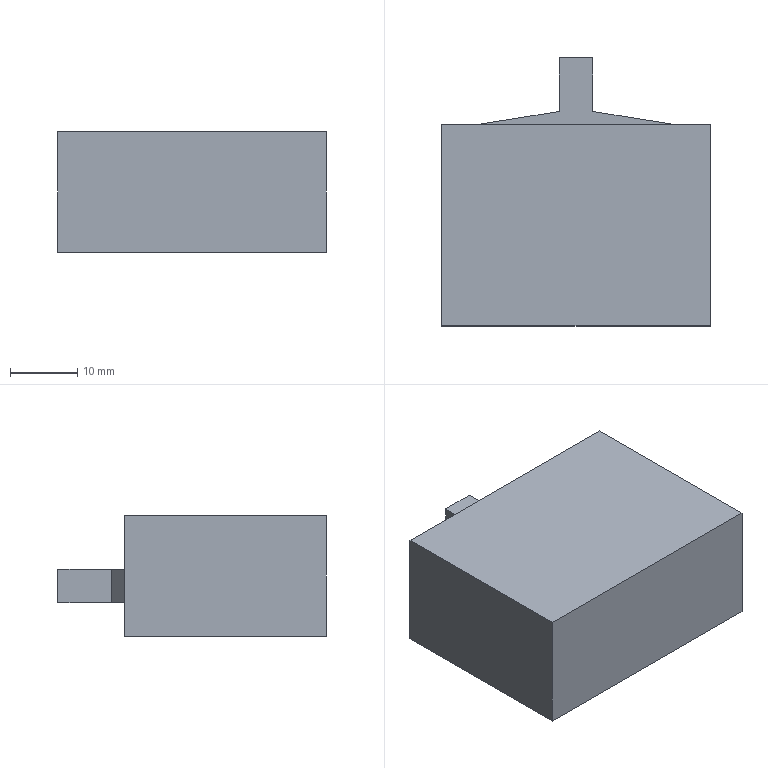Part | SolidWorks | features Extrusion 1, ICE 1 | 1 solid | 13 faces | box 40 x 40 x 18 mm | volume 21975 mm3 | plane 13
STEP:
#1=CARTESIAN_POINT('',(0.,0.,0.));
#2=VERTEX_POINT('',#1);
#3=CARTESIAN_POINT('',(0.,-30.,0.));
#4=VERTEX_POINT('',#3);
#5=CARTESIAN_POINT('',(0.,0.,0.));
#6=DIRECTION('',(0.,-1.,0.));
#7=VECTOR('',#6,1000.);
#8=LINE('',#5,#7);
#9=EDGE_CURVE('',#2,#4,#8,.T.);
#10=ORIENTED_EDGE('',*,*,#9,.T.);
#11=CARTESIAN_POINT('',(0.,-30.,18.));
#12=VERTEX_POINT('',#11);
#13=CARTESIAN_POINT('',(0.,-30.,18.));
#14=DIRECTION('',(0.,0.,-1.));
#15=VECTOR('',#14,1000.);
#16=LINE('',#13,#15);
#17=EDGE_CURVE('',#12,#4,#16,.T.);
#18=ORIENTED_EDGE('',*,*,#17,.F.);
#19=CARTESIAN_POINT('',(0.,0.,18.));
#20=VERTEX_POINT('',#19);
#21=CARTESIAN_POINT('',(0.,0.,18.));
#22=DIRECTION('',(0.,-1.,0.));
#23=VECTOR('',#22,1000.);
#24=LINE('',#21,#23);
#25=EDGE_CURVE('',#20,#12,#24,.T.);
#26=ORIENTED_EDGE('',*,*,#25,.F.);
#27=CARTESIAN_POINT('',(0.,0.,18.));
#28=DIRECTION('',(0.,0.,-1.));
#29=VECTOR('',#28,1000.);
#30=LINE('',#27,#29);
#31=EDGE_CURVE('',#20,#2,#30,.T.);
#32=ORIENTED_EDGE('',*,*,#31,.T.);
#33=EDGE_LOOP('',(#10,#18,#26,#32));
#34=FACE_OUTER_BOUND('',#33,.T.);
#35=CARTESIAN_POINT('',(0.,0.,18.));
#36=DIRECTION('',(1.,0.,0.));
#37=DIRECTION('',(0.,1.,0.));
#38=AXIS2_PLACEMENT_3D('',#35,#36,#37);
#39=PLANE('',#38);
#40=ADVANCED_FACE('',(#34),#39,.F.);
#41=CARTESIAN_POINT('',(40.,-30.,0.));
#42=VERTEX_POINT('',#41);
#43=CARTESIAN_POINT('',(0.,-30.,0.));
#44=DIRECTION('',(1.,0.,0.));
#45=VECTOR('',#44,1000.);
#46=LINE('',#43,#45);
#47=EDGE_CURVE('',#4,#42,#46,.T.);
#48=ORIENTED_EDGE('',*,*,#47,.T.);
#49=CARTESIAN_POINT('',(40.,-30.,18.));
#50=VERTEX_POINT('',#49);
#51=CARTESIAN_POINT('',(40.,-30.,18.));
#52=DIRECTION('',(0.,0.,-1.));
#53=VECTOR('',#52,1000.);
#54=LINE('',#51,#53);
#55=EDGE_CURVE('',#50,#42,#54,.T.);
#56=ORIENTED_EDGE('',*,*,#55,.F.);
#57=CARTESIAN_POINT('',(0.,-30.,18.));
#58=DIRECTION('',(1.,0.,0.));
#59=VECTOR('',#58,1000.);
#60=LINE('',#57,#59);
#61=EDGE_CURVE('',#12,#50,#60,.T.);
#62=ORIENTED_EDGE('',*,*,#61,.F.);
#63=ORIENTED_EDGE('',*,*,#17,.T.);
#64=EDGE_LOOP('',(#48,#56,#62,#63));
#65=FACE_OUTER_BOUND('',#64,.T.);
#66=CARTESIAN_POINT('',(0.,-30.,18.));
#67=DIRECTION('',(0.,1.,0.));
#68=DIRECTION('',(0.,0.,1.));
#69=AXIS2_PLACEMENT_3D('',#66,#67,#68);
#70=PLANE('',#69);
#71=ADVANCED_FACE('',(#65),#70,.F.);
#72=CARTESIAN_POINT('',(40.,0.,0.));
#73=VERTEX_POINT('',#72);
#74=CARTESIAN_POINT('',(40.,0.,0.));
#75=DIRECTION('',(0.,1.,0.));
#76=VECTOR('',#75,1000.);
#77=LINE('',#74,#76);
#78=EDGE_CURVE('',#42,#73,#77,.T.);
#79=ORIENTED_EDGE('',*,*,#78,.T.);
#80=CARTESIAN_POINT('',(40.,0.,18.));
#81=VERTEX_POINT('',#80);
#82=CARTESIAN_POINT('',(40.,0.,18.));
#83=DIRECTION('',(0.,0.,-1.));
#84=VECTOR('',#83,1000.);
#85=LINE('',#82,#84);
#86=EDGE_CURVE('',#81,#73,#85,.T.);
#87=ORIENTED_EDGE('',*,*,#86,.F.);
#88=CARTESIAN_POINT('',(40.,0.,18.));
#89=DIRECTION('',(0.,1.,0.));
#90=VECTOR('',#89,1000.);
#91=LINE('',#88,#90);
#92=EDGE_CURVE('',#50,#81,#91,.T.);
#93=ORIENTED_EDGE('',*,*,#92,.F.);
#94=ORIENTED_EDGE('',*,*,#55,.T.);
#95=EDGE_LOOP('',(#79,#87,#93,#94));
#96=FACE_OUTER_BOUND('',#95,.T.);
#97=CARTESIAN_POINT('',(40.,0.,18.));
#98=DIRECTION('',(-1.,0.,0.));
#99=DIRECTION('',(0.,-1.,0.));
#100=AXIS2_PLACEMENT_3D('',#97,#98,#99);
#101=PLANE('',#100);
#102=ADVANCED_FACE('',(#96),#101,.F.);
#103=CARTESIAN_POINT('',(5.,0.,10.));
#104=VERTEX_POINT('',#103);
#105=CARTESIAN_POINT('',(5.,0.,5.));
#106=VERTEX_POINT('',#105);
#107=CARTESIAN_POINT('',(5.,0.,10.));
#108=DIRECTION('',(0.,0.,-1.));
#109=VECTOR('',#108,1000.);
#110=LINE('',#107,#109);
#111=EDGE_CURVE('',#104,#106,#110,.T.);
#112=ORIENTED_EDGE('',*,*,#111,.T.);
#113=CARTESIAN_POINT('',(35.,0.,5.));
#114=VERTEX_POINT('',#113);
#115=CARTESIAN_POINT('',(0.,0.,5.));
#116=DIRECTION('',(1.,0.,0.));
#117=VECTOR('',#116,1000.);
#118=LINE('',#115,#117);
#119=EDGE_CURVE('',#106,#114,#118,.T.);
#120=ORIENTED_EDGE('',*,*,#119,.T.);
#121=CARTESIAN_POINT('',(35.,0.,10.));
#122=VERTEX_POINT('',#121);
#123=CARTESIAN_POINT('',(35.,0.,10.));
#124=DIRECTION('',(0.,0.,-1.));
#125=VECTOR('',#124,1000.);
#126=LINE('',#123,#125);
#127=EDGE_CURVE('',#122,#114,#126,.T.);
#128=ORIENTED_EDGE('',*,*,#127,.F.);
#129=CARTESIAN_POINT('',(0.,0.,10.));
#130=DIRECTION('',(1.,0.,0.));
#131=VECTOR('',#130,1000.);
#132=LINE('',#129,#131);
#133=EDGE_CURVE('',#104,#122,#132,.T.);
#134=ORIENTED_EDGE('',*,*,#133,.F.);
#135=EDGE_LOOP('',(#112,#120,#128,#134));
#136=FACE_BOUND('',#135,.T.);
#137=CARTESIAN_POINT('',(0.,0.,0.));
#138=DIRECTION('',(-1.,0.,0.));
#139=VECTOR('',#138,1000.);
#140=LINE('',#137,#139);
#141=EDGE_CURVE('',#73,#2,#140,.T.);
#142=ORIENTED_EDGE('',*,*,#141,.T.);
#143=ORIENTED_EDGE('',*,*,#31,.F.);
#144=CARTESIAN_POINT('',(0.,0.,18.));
#145=DIRECTION('',(-1.,0.,0.));
#146=VECTOR('',#145,1000.);
#147=LINE('',#144,#146);
#148=EDGE_CURVE('',#81,#20,#147,.T.);
#149=ORIENTED_EDGE('',*,*,#148,.F.);
#150=ORIENTED_EDGE('',*,*,#86,.T.);
#151=EDGE_LOOP('',(#142,#143,#149,#150));
#152=FACE_OUTER_BOUND('',#151,.T.);
#153=CARTESIAN_POINT('',(0.,0.,18.));
#154=DIRECTION('',(0.,-1.,0.));
#155=DIRECTION('',(0.,0.,-1.));
#156=AXIS2_PLACEMENT_3D('',#153,#154,#155);
#157=PLANE('',#156);
#158=ADVANCED_FACE('',(#136,#152),#157,.F.);
#159=ORIENTED_EDGE('',*,*,#25,.T.);
#160=ORIENTED_EDGE('',*,*,#61,.T.);
#161=ORIENTED_EDGE('',*,*,#92,.T.);
#162=ORIENTED_EDGE('',*,*,#148,.T.);
#163=EDGE_LOOP('',(#159,#160,#161,#162));
#164=FACE_OUTER_BOUND('',#163,.T.);
#165=CARTESIAN_POINT('',(0.,0.,18.));
#166=DIRECTION('',(0.,0.,1.));
#167=DIRECTION('',(1.,0.,0.));
#168=AXIS2_PLACEMENT_3D('',#165,#166,#167);
#169=PLANE('',#168);
#170=ADVANCED_FACE('',(#164),#169,.T.);
#171=ORIENTED_EDGE('',*,*,#9,.F.);
#172=ORIENTED_EDGE('',*,*,#141,.F.);
#173=ORIENTED_EDGE('',*,*,#78,.F.);
#174=ORIENTED_EDGE('',*,*,#47,.F.);
#175=EDGE_LOOP('',(#171,#172,#173,#174));
#176=FACE_OUTER_BOUND('',#175,.T.);
#177=CARTESIAN_POINT('',(0.,0.,0.));
#178=DIRECTION('',(0.,0.,1.));
#179=DIRECTION('',(1.,0.,0.));
#180=AXIS2_PLACEMENT_3D('',#177,#178,#179);
#181=PLANE('',#180);
#182=ADVANCED_FACE('',(#176),#181,.F.);
#183=CARTESIAN_POINT('',(17.5,2.,5.));
#184=VERTEX_POINT('',#183);
#185=CARTESIAN_POINT('',(0.1248,-0.78,5.));
#186=DIRECTION('',(-0.9874,-0.158,0.));
#187=VECTOR('',#186,1000.);
#188=LINE('',#185,#187);
#189=EDGE_CURVE('',#184,#106,#188,.T.);
#190=ORIENTED_EDGE('',*,*,#189,.T.);
#191=ORIENTED_EDGE('',*,*,#111,.F.);
#192=CARTESIAN_POINT('',(17.5,2.,10.));
#193=VERTEX_POINT('',#192);
#194=CARTESIAN_POINT('',(0.1248,-0.78,10.));
#195=DIRECTION('',(-0.9874,-0.158,0.));
#196=VECTOR('',#195,1000.);
#197=LINE('',#194,#196);
#198=EDGE_CURVE('',#193,#104,#197,.T.);
#199=ORIENTED_EDGE('',*,*,#198,.F.);
#200=CARTESIAN_POINT('',(17.5,2.,10.));
#201=DIRECTION('',(0.,0.,-1.));
#202=VECTOR('',#201,1000.);
#203=LINE('',#200,#202);
#204=EDGE_CURVE('',#193,#184,#203,.T.);
#205=ORIENTED_EDGE('',*,*,#204,.T.);
#206=EDGE_LOOP('',(#190,#191,#199,#205));
#207=FACE_OUTER_BOUND('',#206,.T.);
#208=CARTESIAN_POINT('',(0.1248,-0.78,10.));
#209=DIRECTION('',(0.158,-0.9874,0.));
#210=DIRECTION('',(0.9874,0.158,0.));
#211=AXIS2_PLACEMENT_3D('',#208,#209,#210);
#212=PLANE('',#211);
#213=ADVANCED_FACE('',(#207),#212,.F.);
#214=CARTESIAN_POINT('',(22.5,2.,5.));
#215=VERTEX_POINT('',#214);
#216=CARTESIAN_POINT('',(0.8736,5.46,5.));
#217=DIRECTION('',(0.9874,-0.158,0.));
#218=VECTOR('',#217,1000.);
#219=LINE('',#216,#218);
#220=EDGE_CURVE('',#215,#114,#219,.T.);
#221=ORIENTED_EDGE('',*,*,#220,.F.);
#222=CARTESIAN_POINT('',(22.5,2.,10.));
#223=VERTEX_POINT('',#222);
#224=CARTESIAN_POINT('',(22.5,2.,10.));
#225=DIRECTION('',(0.,0.,-1.));
#226=VECTOR('',#225,1000.);
#227=LINE('',#224,#226);
#228=EDGE_CURVE('',#223,#215,#227,.T.);
#229=ORIENTED_EDGE('',*,*,#228,.F.);
#230=CARTESIAN_POINT('',(0.8736,5.46,10.));
#231=DIRECTION('',(0.9874,-0.158,0.));
#232=VECTOR('',#231,1000.);
#233=LINE('',#230,#232);
#234=EDGE_CURVE('',#223,#122,#233,.T.);
#235=ORIENTED_EDGE('',*,*,#234,.T.);
#236=ORIENTED_EDGE('',*,*,#127,.T.);
#237=EDGE_LOOP('',(#221,#229,#235,#236));
#238=FACE_OUTER_BOUND('',#237,.T.);
#239=CARTESIAN_POINT('',(0.8736,5.46,10.));
#240=DIRECTION('',(0.158,0.9874,0.));
#241=DIRECTION('',(-0.9874,0.158,0.));
#242=AXIS2_PLACEMENT_3D('',#239,#240,#241);
#243=PLANE('',#242);
#244=ADVANCED_FACE('',(#238),#243,.T.);
#245=CARTESIAN_POINT('',(22.5,10.,5.));
#246=VERTEX_POINT('',#245);
#247=CARTESIAN_POINT('',(22.5,0.,5.));
#248=DIRECTION('',(0.,1.,0.));
#249=VECTOR('',#248,1000.);
#250=LINE('',#247,#249);
#251=EDGE_CURVE('',#215,#246,#250,.T.);
#252=ORIENTED_EDGE('',*,*,#251,.T.);
#253=CARTESIAN_POINT('',(22.5,10.,10.));
#254=VERTEX_POINT('',#253);
#255=CARTESIAN_POINT('',(22.5,10.,10.));
#256=DIRECTION('',(0.,0.,-1.));
#257=VECTOR('',#256,1000.);
#258=LINE('',#255,#257);
#259=EDGE_CURVE('',#254,#246,#258,.T.);
#260=ORIENTED_EDGE('',*,*,#259,.F.);
#261=CARTESIAN_POINT('',(22.5,0.,10.));
#262=DIRECTION('',(0.,1.,0.));
#263=VECTOR('',#262,1000.);
#264=LINE('',#261,#263);
#265=EDGE_CURVE('',#223,#254,#264,.T.);
#266=ORIENTED_EDGE('',*,*,#265,.F.);
#267=ORIENTED_EDGE('',*,*,#228,.T.);
#268=EDGE_LOOP('',(#252,#260,#266,#267));
#269=FACE_OUTER_BOUND('',#268,.T.);
#270=CARTESIAN_POINT('',(22.5,0.,10.));
#271=DIRECTION('',(-1.,0.,0.));
#272=DIRECTION('',(0.,-1.,0.));
#273=AXIS2_PLACEMENT_3D('',#270,#271,#272);
#274=PLANE('',#273);
#275=ADVANCED_FACE('',(#269),#274,.F.);
#276=CARTESIAN_POINT('',(17.5,10.,5.));
#277=VERTEX_POINT('',#276);
#278=CARTESIAN_POINT('',(0.,10.,5.));
#279=DIRECTION('',(-1.,0.,0.));
#280=VECTOR('',#279,1000.);
#281=LINE('',#278,#280);
#282=EDGE_CURVE('',#246,#277,#281,.T.);
#283=ORIENTED_EDGE('',*,*,#282,.T.);
#284=CARTESIAN_POINT('',(17.5,10.,10.));
#285=VERTEX_POINT('',#284);
#286=CARTESIAN_POINT('',(17.5,10.,10.));
#287=DIRECTION('',(0.,0.,-1.));
#288=VECTOR('',#287,1000.);
#289=LINE('',#286,#288);
#290=EDGE_CURVE('',#285,#277,#289,.T.);
#291=ORIENTED_EDGE('',*,*,#290,.F.);
#292=CARTESIAN_POINT('',(0.,10.,10.));
#293=DIRECTION('',(-1.,0.,0.));
#294=VECTOR('',#293,1000.);
#295=LINE('',#292,#294);
#296=EDGE_CURVE('',#254,#285,#295,.T.);
#297=ORIENTED_EDGE('',*,*,#296,.F.);
#298=ORIENTED_EDGE('',*,*,#259,.T.);
#299=EDGE_LOOP('',(#283,#291,#297,#298));
#300=FACE_OUTER_BOUND('',#299,.T.);
#301=CARTESIAN_POINT('',(0.,10.,10.));
#302=DIRECTION('',(0.,-1.,0.));
#303=DIRECTION('',(0.,0.,-1.));
#304=AXIS2_PLACEMENT_3D('',#301,#302,#303);
#305=PLANE('',#304);
#306=ADVANCED_FACE('',(#300),#305,.F.);
#307=CARTESIAN_POINT('',(17.5,0.,5.));
#308=DIRECTION('',(0.,-1.,0.));
#309=VECTOR('',#308,1000.);
#310=LINE('',#307,#309);
#311=EDGE_CURVE('',#277,#184,#310,.T.);
#312=ORIENTED_EDGE('',*,*,#311,.T.);
#313=ORIENTED_EDGE('',*,*,#204,.F.);
#314=CARTESIAN_POINT('',(17.5,0.,10.));
#315=DIRECTION('',(0.,-1.,0.));
#316=VECTOR('',#315,1000.);
#317=LINE('',#314,#316);
#318=EDGE_CURVE('',#285,#193,#317,.T.);
#319=ORIENTED_EDGE('',*,*,#318,.F.);
#320=ORIENTED_EDGE('',*,*,#290,.T.);
#321=EDGE_LOOP('',(#312,#313,#319,#320));
#322=FACE_OUTER_BOUND('',#321,.T.);
#323=CARTESIAN_POINT('',(17.5,0.,10.));
#324=DIRECTION('',(1.,0.,0.));
#325=DIRECTION('',(0.,1.,0.));
#326=AXIS2_PLACEMENT_3D('',#323,#324,#325);
#327=PLANE('',#326);
#328=ADVANCED_FACE('',(#322),#327,.F.);
#329=ORIENTED_EDGE('',*,*,#198,.T.);
#330=ORIENTED_EDGE('',*,*,#133,.T.);
#331=ORIENTED_EDGE('',*,*,#234,.F.);
#332=ORIENTED_EDGE('',*,*,#265,.T.);
#333=ORIENTED_EDGE('',*,*,#296,.T.);
#334=ORIENTED_EDGE('',*,*,#318,.T.);
#335=EDGE_LOOP('',(#329,#330,#331,#332,#333,#334));
#336=FACE_OUTER_BOUND('',#335,.T.);
#337=CARTESIAN_POINT('',(0.,0.,10.));
#338=DIRECTION('',(0.,0.,-1.));
#339=DIRECTION('',(-1.,0.,0.));
#340=AXIS2_PLACEMENT_3D('',#337,#338,#339);
#341=PLANE('',#340);
#342=ADVANCED_FACE('',(#336),#341,.F.);
#343=ORIENTED_EDGE('',*,*,#189,.F.);
#344=ORIENTED_EDGE('',*,*,#311,.F.);
#345=ORIENTED_EDGE('',*,*,#282,.F.);
#346=ORIENTED_EDGE('',*,*,#251,.F.);
#347=ORIENTED_EDGE('',*,*,#220,.T.);
#348=ORIENTED_EDGE('',*,*,#119,.F.);
#349=EDGE_LOOP('',(#343,#344,#345,#346,#347,#348));
#350=FACE_OUTER_BOUND('',#349,.T.);
#351=CARTESIAN_POINT('',(0.,0.,5.));
#352=DIRECTION('',(0.,0.,-1.));
#353=DIRECTION('',(-1.,0.,0.));
#354=AXIS2_PLACEMENT_3D('',#351,#352,#353);
#355=PLANE('',#354);
#356=ADVANCED_FACE('',(#350),#355,.T.);
#357=CLOSED_SHELL('',(#40,#71,#102,#158,#170,#182,#213,#244,#275,#306,#328,#342,#356));
#358=MANIFOLD_SOLID_BREP('',#357);
#359=CARTESIAN_POINT('',(0.,0.,0.));
#360=DIRECTION('',(0.,0.,1.));
#361=DIRECTION('',(1.,0.,0.));
#362=AXIS2_PLACEMENT_3D('',#359,#360,#361);
#363=(LENGTH_UNIT()NAMED_UNIT(*)SI_UNIT(.MILLI.,.METRE.));
#364=UNCERTAINTY_MEASURE_WITH_UNIT(LENGTH_MEASURE(0.00001),#363,'','');
#365=(NAMED_UNIT(*)PLANE_ANGLE_UNIT()SI_UNIT($,.RADIAN.));
#366=(NAMED_UNIT(*)SI_UNIT($,.STERADIAN.)SOLID_ANGLE_UNIT());
#367=(GEOMETRIC_REPRESENTATION_CONTEXT(3)GLOBAL_UNCERTAINTY_ASSIGNED_CONTEXT((#364))GLOBAL_UNIT_ASSIGNED_CONTEXT((#363,#365,#366))REPRESENTATION_CONTEXT('',''));
#368=ADVANCED_BREP_SHAPE_REPRESENTATION('',(#358,#362),#367);